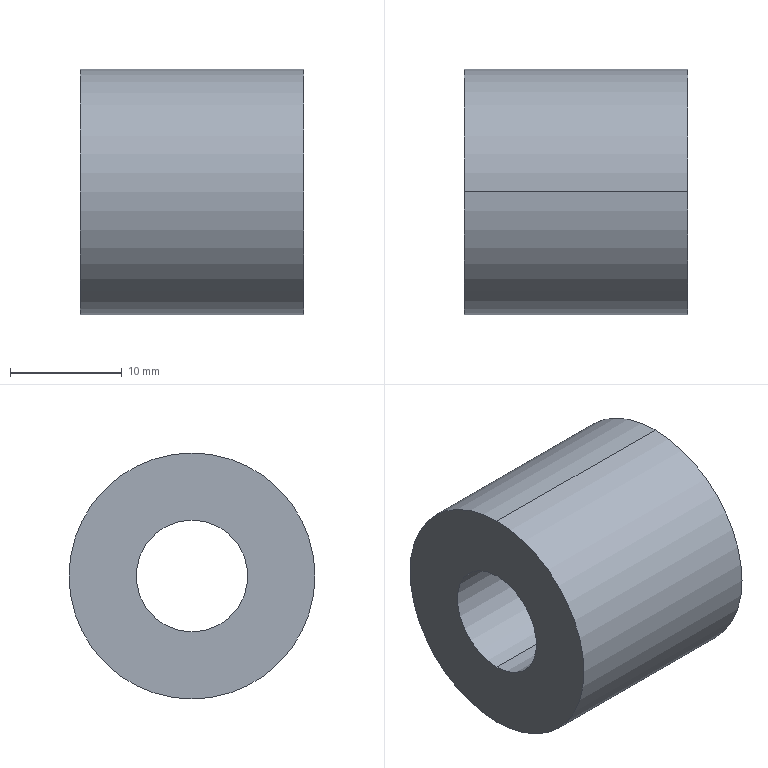Part | SolidWorks | features BaseBody 1 | 1 solid | 6 faces | box 20 x 22 x 22 mm | volume 6032 mm3 | cylinder 4 | plane 2 | commonest cylinder face diameters 10 x2 22 x2
STEP:
#1=CARTESIAN_POINT('',(-114.,-57.,68.));
#2=VERTEX_POINT('',#1);
#3=CARTESIAN_POINT('',(-114.,-57.,46.));
#4=VERTEX_POINT('',#3);
#5=CARTESIAN_POINT('',(-114.,-57.,57.));
#6=DIRECTION('',(-1.,0.,0.));
#7=DIRECTION('',(0.,0.,1.));
#8=AXIS2_PLACEMENT_3D('',#5,#6,#7);
#9=CIRCLE('',#8,11.);
#10=EDGE_CURVE('',#2,#4,#9,.T.);
#11=ORIENTED_EDGE('',*,*,#10,.T.);
#12=CARTESIAN_POINT('',(-134.,-57.,46.));
#13=VERTEX_POINT('',#12);
#14=CARTESIAN_POINT('',(-114.,-57.,46.));
#15=DIRECTION('',(-1.,0.,0.));
#16=VECTOR('',#15,1000.);
#17=LINE('',#14,#16);
#18=EDGE_CURVE('',#4,#13,#17,.T.);
#19=ORIENTED_EDGE('',*,*,#18,.T.);
#20=CARTESIAN_POINT('',(-134.,-57.,68.));
#21=VERTEX_POINT('',#20);
#22=CARTESIAN_POINT('',(-134.,-57.,57.));
#23=DIRECTION('',(1.,0.,0.));
#24=DIRECTION('',(0.,0.,1.));
#25=AXIS2_PLACEMENT_3D('',#22,#23,#24);
#26=CIRCLE('',#25,11.);
#27=EDGE_CURVE('',#13,#21,#26,.T.);
#28=ORIENTED_EDGE('',*,*,#27,.T.);
#29=CARTESIAN_POINT('',(-114.,-57.,68.));
#30=DIRECTION('',(-1.,0.,0.));
#31=VECTOR('',#30,1000.);
#32=LINE('',#29,#31);
#33=EDGE_CURVE('',#2,#21,#32,.T.);
#34=ORIENTED_EDGE('',*,*,#33,.F.);
#35=EDGE_LOOP('',(#11,#19,#28,#34));
#36=FACE_OUTER_BOUND('',#35,.T.);
#37=CARTESIAN_POINT('',(-114.,-57.,57.));
#38=DIRECTION('',(-1.,0.,0.));
#39=DIRECTION('',(0.,0.,1.));
#40=AXIS2_PLACEMENT_3D('',#37,#38,#39);
#41=CYLINDRICAL_SURFACE('',#40,11.);
#42=ADVANCED_FACE('',(#36),#41,.T.);
#43=CARTESIAN_POINT('',(-114.,-57.,52.));
#44=VERTEX_POINT('',#43);
#45=CARTESIAN_POINT('',(-114.,-57.,62.));
#46=VERTEX_POINT('',#45);
#47=CARTESIAN_POINT('',(-114.,-57.,57.));
#48=DIRECTION('',(-1.,0.,0.));
#49=DIRECTION('',(0.,0.,1.));
#50=AXIS2_PLACEMENT_3D('',#47,#48,#49);
#51=CIRCLE('',#50,5.);
#52=EDGE_CURVE('',#44,#46,#51,.T.);
#53=ORIENTED_EDGE('',*,*,#52,.F.);
#54=CARTESIAN_POINT('',(-134.,-57.,52.));
#55=VERTEX_POINT('',#54);
#56=CARTESIAN_POINT('',(-114.,-57.,52.));
#57=DIRECTION('',(-1.,0.,0.));
#58=VECTOR('',#57,1000.);
#59=LINE('',#56,#58);
#60=EDGE_CURVE('',#44,#55,#59,.T.);
#61=ORIENTED_EDGE('',*,*,#60,.T.);
#62=CARTESIAN_POINT('',(-134.,-57.,62.));
#63=VERTEX_POINT('',#62);
#64=CARTESIAN_POINT('',(-134.,-57.,57.));
#65=DIRECTION('',(-1.,0.,0.));
#66=DIRECTION('',(0.,0.,1.));
#67=AXIS2_PLACEMENT_3D('',#64,#65,#66);
#68=CIRCLE('',#67,5.);
#69=EDGE_CURVE('',#55,#63,#68,.T.);
#70=ORIENTED_EDGE('',*,*,#69,.T.);
#71=CARTESIAN_POINT('',(-114.,-57.,62.));
#72=DIRECTION('',(-1.,0.,0.));
#73=VECTOR('',#72,1000.);
#74=LINE('',#71,#73);
#75=EDGE_CURVE('',#46,#63,#74,.T.);
#76=ORIENTED_EDGE('',*,*,#75,.F.);
#77=EDGE_LOOP('',(#53,#61,#70,#76));
#78=FACE_OUTER_BOUND('',#77,.T.);
#79=CARTESIAN_POINT('',(-114.,-57.,57.));
#80=DIRECTION('',(-1.,0.,0.));
#81=DIRECTION('',(0.,0.,1.));
#82=AXIS2_PLACEMENT_3D('',#79,#80,#81);
#83=CYLINDRICAL_SURFACE('',#82,5.);
#84=ADVANCED_FACE('',(#78),#83,.F.);
#85=ORIENTED_EDGE('',*,*,#18,.F.);
#86=CARTESIAN_POINT('',(-114.,-57.,57.));
#87=DIRECTION('',(-1.,0.,0.));
#88=DIRECTION('',(0.,0.,1.));
#89=AXIS2_PLACEMENT_3D('',#86,#87,#88);
#90=CIRCLE('',#89,11.);
#91=EDGE_CURVE('',#4,#2,#90,.T.);
#92=ORIENTED_EDGE('',*,*,#91,.T.);
#93=ORIENTED_EDGE('',*,*,#33,.T.);
#94=CARTESIAN_POINT('',(-134.,-57.,57.));
#95=DIRECTION('',(1.,0.,0.));
#96=DIRECTION('',(0.,0.,1.));
#97=AXIS2_PLACEMENT_3D('',#94,#95,#96);
#98=CIRCLE('',#97,11.);
#99=EDGE_CURVE('',#21,#13,#98,.T.);
#100=ORIENTED_EDGE('',*,*,#99,.T.);
#101=EDGE_LOOP('',(#85,#92,#93,#100));
#102=FACE_OUTER_BOUND('',#101,.T.);
#103=CARTESIAN_POINT('',(-114.,-57.,57.));
#104=DIRECTION('',(-1.,0.,0.));
#105=DIRECTION('',(0.,0.,1.));
#106=AXIS2_PLACEMENT_3D('',#103,#104,#105);
#107=CYLINDRICAL_SURFACE('',#106,11.);
#108=ADVANCED_FACE('',(#102),#107,.T.);
#109=CARTESIAN_POINT('',(-114.,-57.,57.));
#110=DIRECTION('',(-1.,0.,0.));
#111=DIRECTION('',(0.,0.,1.));
#112=AXIS2_PLACEMENT_3D('',#109,#110,#111);
#113=CIRCLE('',#112,5.);
#114=EDGE_CURVE('',#46,#44,#113,.T.);
#115=ORIENTED_EDGE('',*,*,#114,.T.);
#116=ORIENTED_EDGE('',*,*,#52,.T.);
#117=EDGE_LOOP('',(#115,#116));
#118=FACE_BOUND('',#117,.T.);
#119=ORIENTED_EDGE('',*,*,#10,.F.);
#120=ORIENTED_EDGE('',*,*,#91,.F.);
#121=EDGE_LOOP('',(#119,#120));
#122=FACE_OUTER_BOUND('',#121,.T.);
#123=CARTESIAN_POINT('',(-114.,-57.,57.));
#124=DIRECTION('',(1.,0.,0.));
#125=DIRECTION('',(0.,0.,-1.));
#126=AXIS2_PLACEMENT_3D('',#123,#124,#125);
#127=PLANE('',#126);
#128=ADVANCED_FACE('',(#118,#122),#127,.T.);
#129=CARTESIAN_POINT('',(-134.,-57.,57.));
#130=DIRECTION('',(-1.,0.,0.));
#131=DIRECTION('',(0.,0.,1.));
#132=AXIS2_PLACEMENT_3D('',#129,#130,#131);
#133=CIRCLE('',#132,5.);
#134=EDGE_CURVE('',#63,#55,#133,.T.);
#135=ORIENTED_EDGE('',*,*,#134,.F.);
#136=ORIENTED_EDGE('',*,*,#69,.F.);
#137=EDGE_LOOP('',(#135,#136));
#138=FACE_BOUND('',#137,.T.);
#139=ORIENTED_EDGE('',*,*,#99,.F.);
#140=ORIENTED_EDGE('',*,*,#27,.F.);
#141=EDGE_LOOP('',(#139,#140));
#142=FACE_OUTER_BOUND('',#141,.T.);
#143=CARTESIAN_POINT('',(-134.,-57.,57.));
#144=DIRECTION('',(1.,0.,0.));
#145=DIRECTION('',(0.,0.,-1.));
#146=AXIS2_PLACEMENT_3D('',#143,#144,#145);
#147=PLANE('',#146);
#148=ADVANCED_FACE('',(#138,#142),#147,.F.);
#149=ORIENTED_EDGE('',*,*,#60,.F.);
#150=ORIENTED_EDGE('',*,*,#114,.F.);
#151=ORIENTED_EDGE('',*,*,#75,.T.);
#152=ORIENTED_EDGE('',*,*,#134,.T.);
#153=EDGE_LOOP('',(#149,#150,#151,#152));
#154=FACE_OUTER_BOUND('',#153,.T.);
#155=CARTESIAN_POINT('',(-114.,-57.,57.));
#156=DIRECTION('',(-1.,0.,0.));
#157=DIRECTION('',(0.,0.,1.));
#158=AXIS2_PLACEMENT_3D('',#155,#156,#157);
#159=CYLINDRICAL_SURFACE('',#158,5.);
#160=ADVANCED_FACE('',(#154),#159,.F.);
#161=CLOSED_SHELL('',(#42,#84,#108,#128,#148,#160));
#162=MANIFOLD_SOLID_BREP('',#161);
#163=CARTESIAN_POINT('',(0.,0.,0.));
#164=DIRECTION('',(0.,0.,1.));
#165=DIRECTION('',(1.,0.,0.));
#166=AXIS2_PLACEMENT_3D('',#163,#164,#165);
#167=(LENGTH_UNIT()NAMED_UNIT(*)SI_UNIT(.MILLI.,.METRE.));
#168=UNCERTAINTY_MEASURE_WITH_UNIT(LENGTH_MEASURE(0.00001),#167,'','');
#169=(NAMED_UNIT(*)PLANE_ANGLE_UNIT()SI_UNIT($,.RADIAN.));
#170=(NAMED_UNIT(*)SI_UNIT($,.STERADIAN.)SOLID_ANGLE_UNIT());
#171=(GEOMETRIC_REPRESENTATION_CONTEXT(3)GLOBAL_UNCERTAINTY_ASSIGNED_CONTEXT((#168))GLOBAL_UNIT_ASSIGNED_CONTEXT((#167,#169,#170))REPRESENTATION_CONTEXT('',''));
#172=ADVANCED_BREP_SHAPE_REPRESENTATION('',(#162,#166),#171);